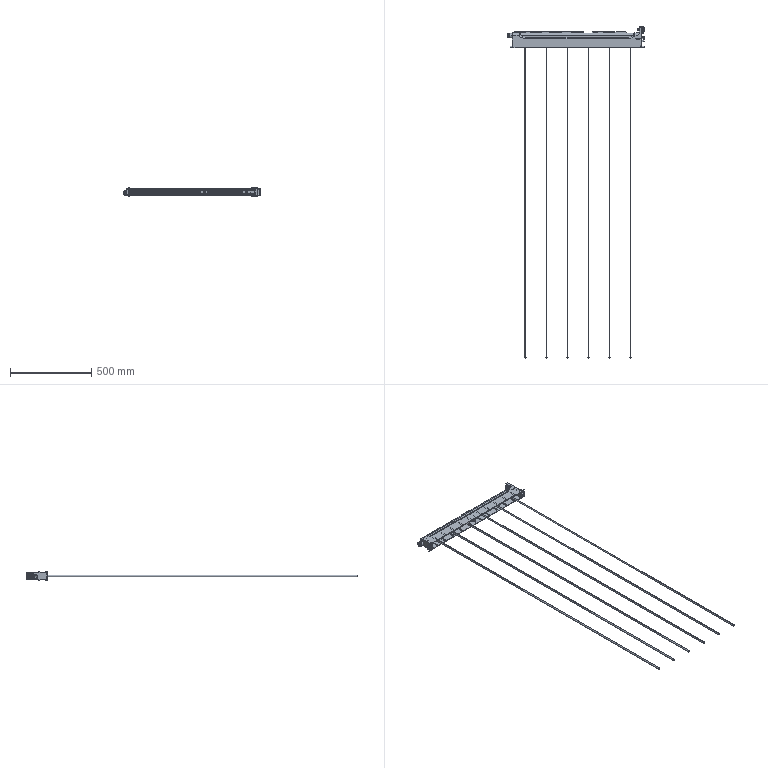Part | SolidWorks | features BaseBody 2, ICE 1 | 2 solids | 728 faces | box 842.8 x 2047 x 56.2 mm | volume 1758530 mm3 | plane 409 | cylinder 171 | spline 87 | torus 35 | cone 26 | commonest cylinder face diameters 1 x60 10 x12 12 x12 22 x9 1.5 x8 3.5 x6